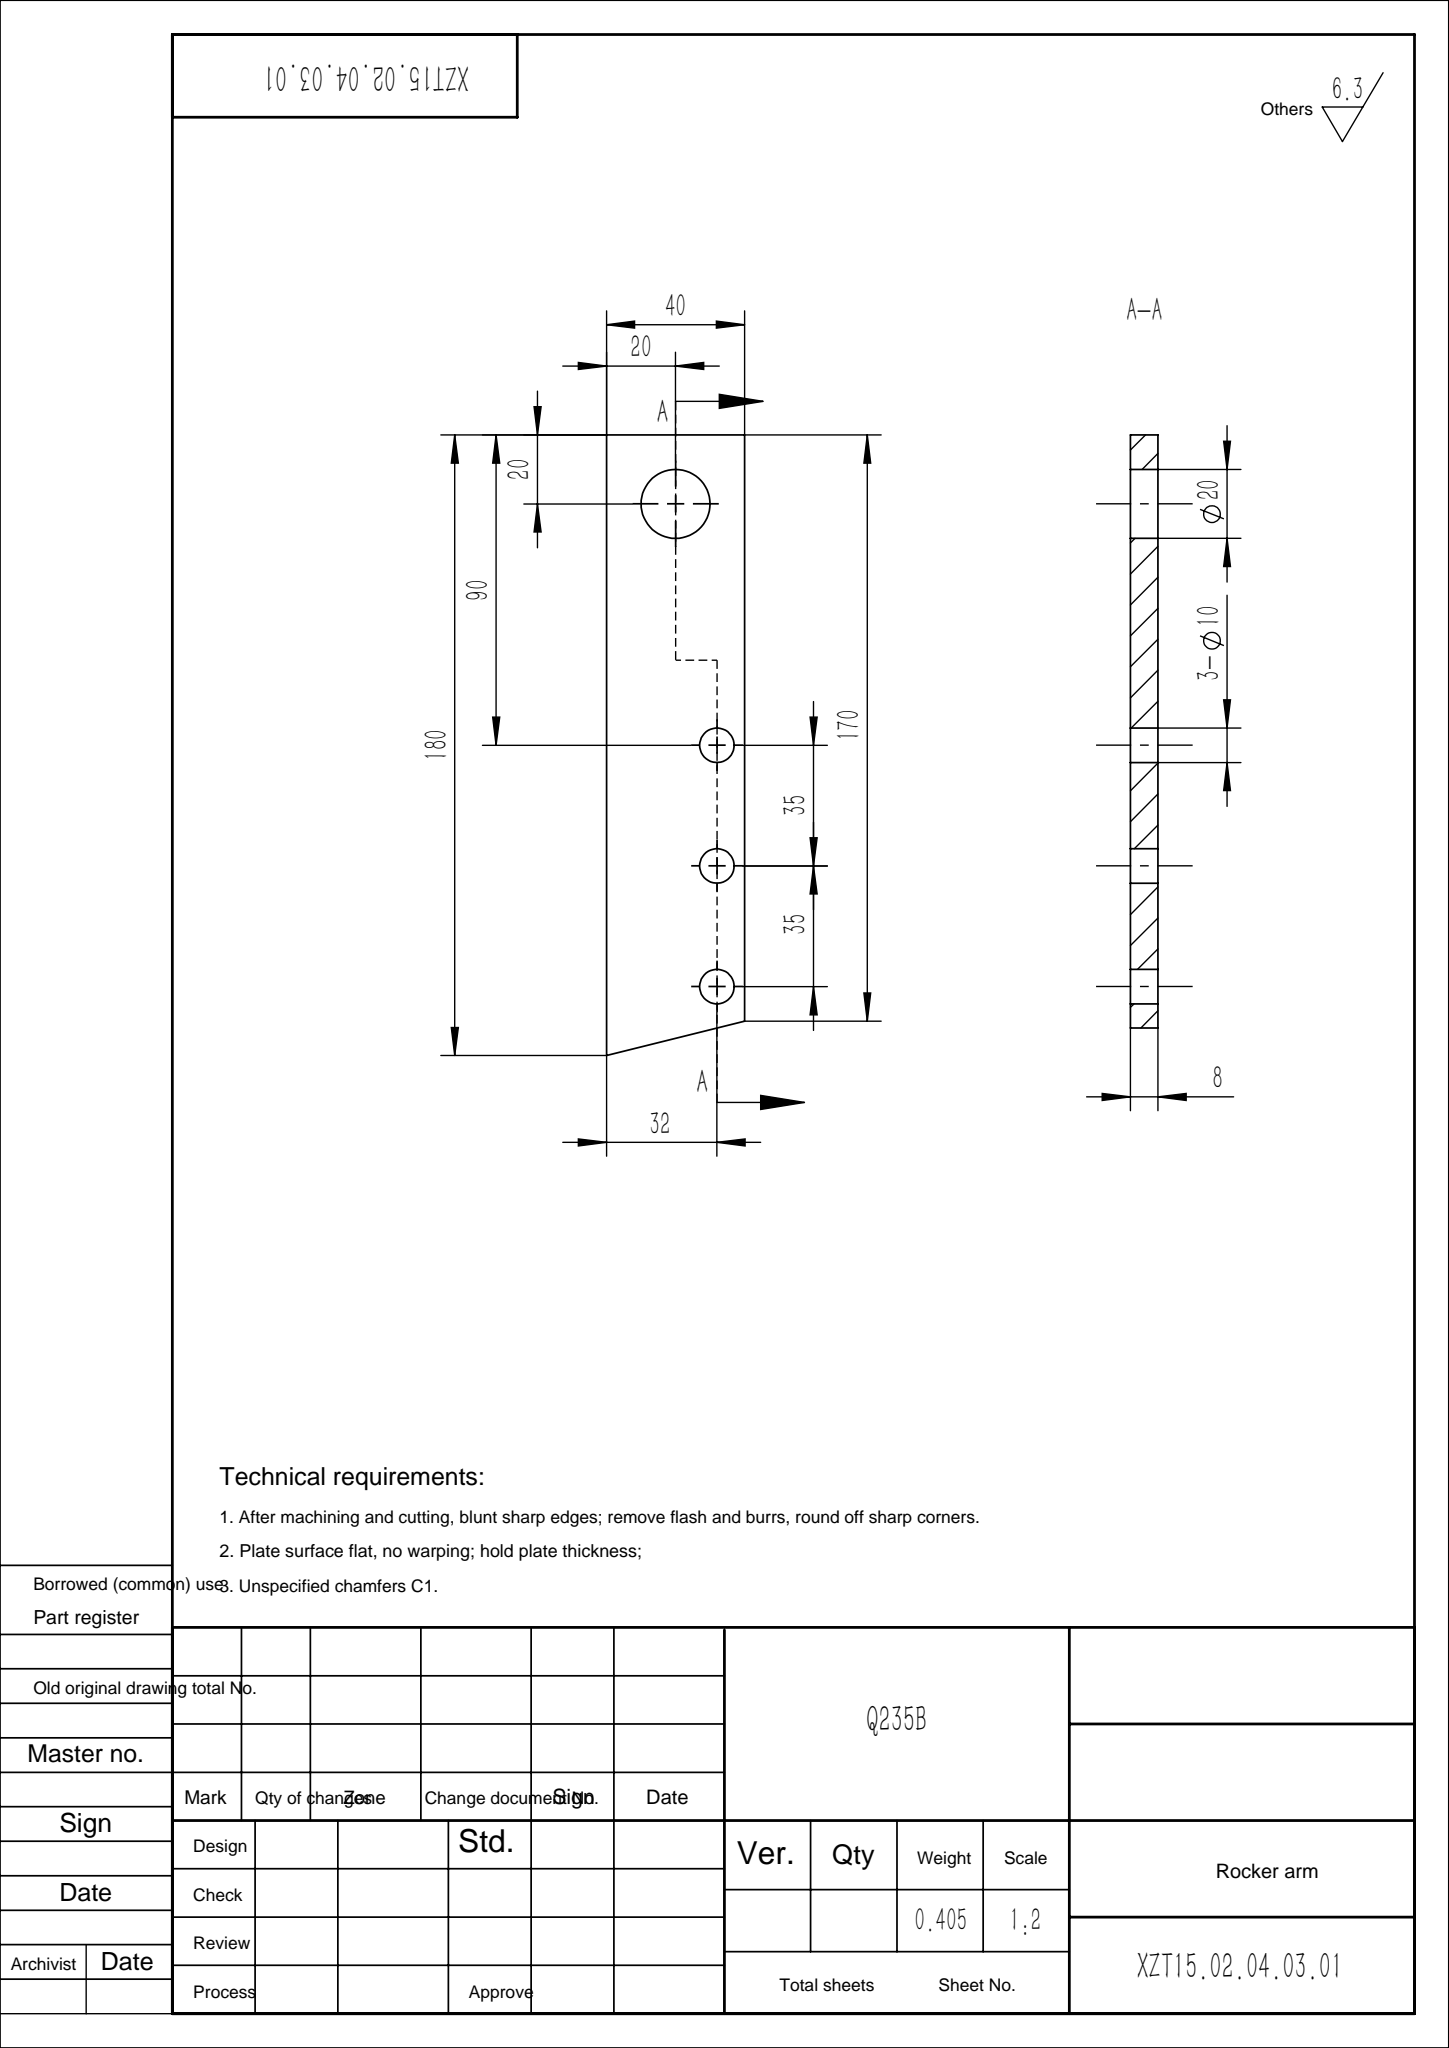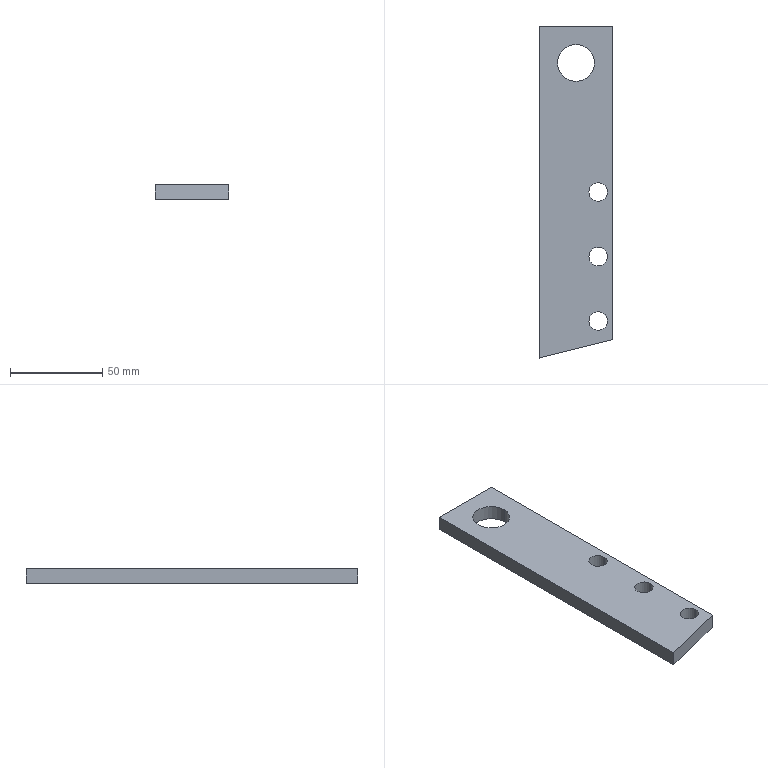Part | SolidWorks | features Extrusion 1 | 1 solid | 14 faces | box 40 x 180 x 8 mm | volume 51602 mm3 | cylinder 8 | plane 6 | commonest cylinder face diameters 10 x6 20 x2
STEP:
#1=CARTESIAN_POINT('',(27.,20.,4.));
#2=VERTEX_POINT('',#1);
#3=CARTESIAN_POINT('',(37.,20.,4.));
#4=VERTEX_POINT('',#3);
#5=CARTESIAN_POINT('',(32.,20.,4.));
#6=DIRECTION('',(0.,0.,1.));
#7=DIRECTION('',(1.,0.,0.));
#8=AXIS2_PLACEMENT_3D('',#5,#6,#7);
#9=CIRCLE('',#8,5.);
#10=EDGE_CURVE('',#2,#4,#9,.T.);
#11=ORIENTED_EDGE('',*,*,#10,.T.);
#12=CARTESIAN_POINT('',(37.,20.,-4.));
#13=VERTEX_POINT('',#12);
#14=CARTESIAN_POINT('',(37.,20.,4.));
#15=DIRECTION('',(0.,0.,-1.));
#16=VECTOR('',#15,1000.);
#17=LINE('',#14,#16);
#18=EDGE_CURVE('',#4,#13,#17,.T.);
#19=ORIENTED_EDGE('',*,*,#18,.T.);
#20=CARTESIAN_POINT('',(27.,20.,-4.));
#21=VERTEX_POINT('',#20);
#22=CARTESIAN_POINT('',(32.,20.,-4.));
#23=DIRECTION('',(0.,0.,1.));
#24=DIRECTION('',(1.,0.,0.));
#25=AXIS2_PLACEMENT_3D('',#22,#23,#24);
#26=CIRCLE('',#25,5.);
#27=EDGE_CURVE('',#21,#13,#26,.T.);
#28=ORIENTED_EDGE('',*,*,#27,.F.);
#29=CARTESIAN_POINT('',(27.,20.,4.));
#30=DIRECTION('',(0.,0.,-1.));
#31=VECTOR('',#30,1000.);
#32=LINE('',#29,#31);
#33=EDGE_CURVE('',#2,#21,#32,.T.);
#34=ORIENTED_EDGE('',*,*,#33,.F.);
#35=EDGE_LOOP('',(#11,#19,#28,#34));
#36=FACE_OUTER_BOUND('',#35,.T.);
#37=CARTESIAN_POINT('',(32.,20.,4.));
#38=DIRECTION('',(0.,0.,-1.));
#39=DIRECTION('',(-1.,0.,0.));
#40=AXIS2_PLACEMENT_3D('',#37,#38,#39);
#41=CYLINDRICAL_SURFACE('',#40,5.);
#42=ADVANCED_FACE('',(#36),#41,.F.);
#43=CARTESIAN_POINT('',(27.,55.,4.));
#44=VERTEX_POINT('',#43);
#45=CARTESIAN_POINT('',(37.,55.,4.));
#46=VERTEX_POINT('',#45);
#47=CARTESIAN_POINT('',(32.,55.,4.));
#48=DIRECTION('',(0.,0.,1.));
#49=DIRECTION('',(1.,0.,0.));
#50=AXIS2_PLACEMENT_3D('',#47,#48,#49);
#51=CIRCLE('',#50,5.);
#52=EDGE_CURVE('',#44,#46,#51,.T.);
#53=ORIENTED_EDGE('',*,*,#52,.T.);
#54=CARTESIAN_POINT('',(37.,55.,-4.));
#55=VERTEX_POINT('',#54);
#56=CARTESIAN_POINT('',(37.,55.,4.));
#57=DIRECTION('',(0.,0.,-1.));
#58=VECTOR('',#57,1000.);
#59=LINE('',#56,#58);
#60=EDGE_CURVE('',#46,#55,#59,.T.);
#61=ORIENTED_EDGE('',*,*,#60,.T.);
#62=CARTESIAN_POINT('',(27.,55.,-4.));
#63=VERTEX_POINT('',#62);
#64=CARTESIAN_POINT('',(32.,55.,-4.));
#65=DIRECTION('',(0.,0.,1.));
#66=DIRECTION('',(1.,0.,0.));
#67=AXIS2_PLACEMENT_3D('',#64,#65,#66);
#68=CIRCLE('',#67,5.);
#69=EDGE_CURVE('',#63,#55,#68,.T.);
#70=ORIENTED_EDGE('',*,*,#69,.F.);
#71=CARTESIAN_POINT('',(27.,55.,4.));
#72=DIRECTION('',(0.,0.,-1.));
#73=VECTOR('',#72,1000.);
#74=LINE('',#71,#73);
#75=EDGE_CURVE('',#44,#63,#74,.T.);
#76=ORIENTED_EDGE('',*,*,#75,.F.);
#77=EDGE_LOOP('',(#53,#61,#70,#76));
#78=FACE_OUTER_BOUND('',#77,.T.);
#79=CARTESIAN_POINT('',(32.,55.,4.));
#80=DIRECTION('',(0.,0.,-1.));
#81=DIRECTION('',(-1.,0.,0.));
#82=AXIS2_PLACEMENT_3D('',#79,#80,#81);
#83=CYLINDRICAL_SURFACE('',#82,5.);
#84=ADVANCED_FACE('',(#78),#83,.F.);
#85=CARTESIAN_POINT('',(27.,90.,4.));
#86=VERTEX_POINT('',#85);
#87=CARTESIAN_POINT('',(37.,90.,4.));
#88=VERTEX_POINT('',#87);
#89=CARTESIAN_POINT('',(32.,90.,4.));
#90=DIRECTION('',(0.,0.,1.));
#91=DIRECTION('',(1.,0.,0.));
#92=AXIS2_PLACEMENT_3D('',#89,#90,#91);
#93=CIRCLE('',#92,5.);
#94=EDGE_CURVE('',#86,#88,#93,.T.);
#95=ORIENTED_EDGE('',*,*,#94,.T.);
#96=CARTESIAN_POINT('',(37.,90.,-4.));
#97=VERTEX_POINT('',#96);
#98=CARTESIAN_POINT('',(37.,90.,4.));
#99=DIRECTION('',(0.,0.,-1.));
#100=VECTOR('',#99,1000.);
#101=LINE('',#98,#100);
#102=EDGE_CURVE('',#88,#97,#101,.T.);
#103=ORIENTED_EDGE('',*,*,#102,.T.);
#104=CARTESIAN_POINT('',(27.,90.,-4.));
#105=VERTEX_POINT('',#104);
#106=CARTESIAN_POINT('',(32.,90.,-4.));
#107=DIRECTION('',(0.,0.,1.));
#108=DIRECTION('',(1.,0.,0.));
#109=AXIS2_PLACEMENT_3D('',#106,#107,#108);
#110=CIRCLE('',#109,5.);
#111=EDGE_CURVE('',#105,#97,#110,.T.);
#112=ORIENTED_EDGE('',*,*,#111,.F.);
#113=CARTESIAN_POINT('',(27.,90.,4.));
#114=DIRECTION('',(0.,0.,-1.));
#115=VECTOR('',#114,1000.);
#116=LINE('',#113,#115);
#117=EDGE_CURVE('',#86,#105,#116,.T.);
#118=ORIENTED_EDGE('',*,*,#117,.F.);
#119=EDGE_LOOP('',(#95,#103,#112,#118));
#120=FACE_OUTER_BOUND('',#119,.T.);
#121=CARTESIAN_POINT('',(32.,90.,4.));
#122=DIRECTION('',(0.,0.,-1.));
#123=DIRECTION('',(-1.,0.,0.));
#124=AXIS2_PLACEMENT_3D('',#121,#122,#123);
#125=CYLINDRICAL_SURFACE('',#124,5.);
#126=ADVANCED_FACE('',(#120),#125,.F.);
#127=CARTESIAN_POINT('',(10.,160.,4.));
#128=VERTEX_POINT('',#127);
#129=CARTESIAN_POINT('',(30.,160.,4.));
#130=VERTEX_POINT('',#129);
#131=CARTESIAN_POINT('',(20.,160.,4.));
#132=DIRECTION('',(0.,0.,1.));
#133=DIRECTION('',(1.,0.,0.));
#134=AXIS2_PLACEMENT_3D('',#131,#132,#133);
#135=CIRCLE('',#134,10.);
#136=EDGE_CURVE('',#128,#130,#135,.T.);
#137=ORIENTED_EDGE('',*,*,#136,.T.);
#138=CARTESIAN_POINT('',(30.,160.,-4.));
#139=VERTEX_POINT('',#138);
#140=CARTESIAN_POINT('',(30.,160.,4.));
#141=DIRECTION('',(0.,0.,-1.));
#142=VECTOR('',#141,1000.);
#143=LINE('',#140,#142);
#144=EDGE_CURVE('',#130,#139,#143,.T.);
#145=ORIENTED_EDGE('',*,*,#144,.T.);
#146=CARTESIAN_POINT('',(10.,160.,-4.));
#147=VERTEX_POINT('',#146);
#148=CARTESIAN_POINT('',(20.,160.,-4.));
#149=DIRECTION('',(0.,0.,1.));
#150=DIRECTION('',(1.,0.,0.));
#151=AXIS2_PLACEMENT_3D('',#148,#149,#150);
#152=CIRCLE('',#151,10.);
#153=EDGE_CURVE('',#147,#139,#152,.T.);
#154=ORIENTED_EDGE('',*,*,#153,.F.);
#155=CARTESIAN_POINT('',(10.,160.,4.));
#156=DIRECTION('',(0.,0.,-1.));
#157=VECTOR('',#156,1000.);
#158=LINE('',#155,#157);
#159=EDGE_CURVE('',#128,#147,#158,.T.);
#160=ORIENTED_EDGE('',*,*,#159,.F.);
#161=EDGE_LOOP('',(#137,#145,#154,#160));
#162=FACE_OUTER_BOUND('',#161,.T.);
#163=CARTESIAN_POINT('',(20.,160.,4.));
#164=DIRECTION('',(0.,0.,-1.));
#165=DIRECTION('',(-1.,0.,0.));
#166=AXIS2_PLACEMENT_3D('',#163,#164,#165);
#167=CYLINDRICAL_SURFACE('',#166,10.);
#168=ADVANCED_FACE('',(#162),#167,.F.);
#169=CARTESIAN_POINT('',(0.,0.,4.));
#170=VERTEX_POINT('',#169);
#171=CARTESIAN_POINT('',(40.,10.,4.));
#172=VERTEX_POINT('',#171);
#173=CARTESIAN_POINT('',(40.,10.,4.));
#174=DIRECTION('',(0.9701,0.2425,0.));
#175=VECTOR('',#174,1000.);
#176=LINE('',#173,#175);
#177=EDGE_CURVE('',#170,#172,#176,.T.);
#178=ORIENTED_EDGE('',*,*,#177,.T.);
#179=CARTESIAN_POINT('',(40.,180.,4.));
#180=VERTEX_POINT('',#179);
#181=CARTESIAN_POINT('',(40.,180.,4.));
#182=DIRECTION('',(0.,1.,0.));
#183=VECTOR('',#182,1000.);
#184=LINE('',#181,#183);
#185=EDGE_CURVE('',#172,#180,#184,.T.);
#186=ORIENTED_EDGE('',*,*,#185,.T.);
#187=CARTESIAN_POINT('',(0.,180.,4.));
#188=VERTEX_POINT('',#187);
#189=CARTESIAN_POINT('',(0.,180.,4.));
#190=DIRECTION('',(-1.,0.,0.));
#191=VECTOR('',#190,1000.);
#192=LINE('',#189,#191);
#193=EDGE_CURVE('',#180,#188,#192,.T.);
#194=ORIENTED_EDGE('',*,*,#193,.T.);
#195=CARTESIAN_POINT('',(0.,0.,4.));
#196=DIRECTION('',(0.,-1.,0.));
#197=VECTOR('',#196,1000.);
#198=LINE('',#195,#197);
#199=EDGE_CURVE('',#188,#170,#198,.T.);
#200=ORIENTED_EDGE('',*,*,#199,.T.);
#201=EDGE_LOOP('',(#178,#186,#194,#200));
#202=FACE_OUTER_BOUND('',#201,.T.);
#203=ORIENTED_EDGE('',*,*,#136,.F.);
#204=CARTESIAN_POINT('',(20.,160.,4.));
#205=DIRECTION('',(0.,0.,1.));
#206=DIRECTION('',(1.,0.,0.));
#207=AXIS2_PLACEMENT_3D('',#204,#205,#206);
#208=CIRCLE('',#207,10.);
#209=EDGE_CURVE('',#130,#128,#208,.T.);
#210=ORIENTED_EDGE('',*,*,#209,.F.);
#211=EDGE_LOOP('',(#203,#210));
#212=FACE_BOUND('',#211,.T.);
#213=ORIENTED_EDGE('',*,*,#94,.F.);
#214=CARTESIAN_POINT('',(32.,90.,4.));
#215=DIRECTION('',(0.,0.,1.));
#216=DIRECTION('',(1.,0.,0.));
#217=AXIS2_PLACEMENT_3D('',#214,#215,#216);
#218=CIRCLE('',#217,5.);
#219=EDGE_CURVE('',#88,#86,#218,.T.);
#220=ORIENTED_EDGE('',*,*,#219,.F.);
#221=EDGE_LOOP('',(#213,#220));
#222=FACE_BOUND('',#221,.T.);
#223=ORIENTED_EDGE('',*,*,#52,.F.);
#224=CARTESIAN_POINT('',(32.,55.,4.));
#225=DIRECTION('',(0.,0.,1.));
#226=DIRECTION('',(1.,0.,0.));
#227=AXIS2_PLACEMENT_3D('',#224,#225,#226);
#228=CIRCLE('',#227,5.);
#229=EDGE_CURVE('',#46,#44,#228,.T.);
#230=ORIENTED_EDGE('',*,*,#229,.F.);
#231=EDGE_LOOP('',(#223,#230));
#232=FACE_BOUND('',#231,.T.);
#233=ORIENTED_EDGE('',*,*,#10,.F.);
#234=CARTESIAN_POINT('',(32.,20.,4.));
#235=DIRECTION('',(0.,0.,1.));
#236=DIRECTION('',(1.,0.,0.));
#237=AXIS2_PLACEMENT_3D('',#234,#235,#236);
#238=CIRCLE('',#237,5.);
#239=EDGE_CURVE('',#4,#2,#238,.T.);
#240=ORIENTED_EDGE('',*,*,#239,.F.);
#241=EDGE_LOOP('',(#233,#240));
#242=FACE_BOUND('',#241,.T.);
#243=CARTESIAN_POINT('',(0.,0.,4.));
#244=DIRECTION('',(0.,0.,-1.));
#245=DIRECTION('',(-1.,0.,0.));
#246=AXIS2_PLACEMENT_3D('',#243,#244,#245);
#247=PLANE('',#246);
#248=ADVANCED_FACE('',(#202,#212,#222,#232,#242),#247,.F.);
#249=ORIENTED_EDGE('',*,*,#69,.T.);
#250=CARTESIAN_POINT('',(32.,55.,-4.));
#251=DIRECTION('',(0.,0.,1.));
#252=DIRECTION('',(1.,0.,0.));
#253=AXIS2_PLACEMENT_3D('',#250,#251,#252);
#254=CIRCLE('',#253,5.);
#255=EDGE_CURVE('',#55,#63,#254,.T.);
#256=ORIENTED_EDGE('',*,*,#255,.T.);
#257=EDGE_LOOP('',(#249,#256));
#258=FACE_BOUND('',#257,.T.);
#259=ORIENTED_EDGE('',*,*,#153,.T.);
#260=CARTESIAN_POINT('',(20.,160.,-4.));
#261=DIRECTION('',(0.,0.,1.));
#262=DIRECTION('',(1.,0.,0.));
#263=AXIS2_PLACEMENT_3D('',#260,#261,#262);
#264=CIRCLE('',#263,10.);
#265=EDGE_CURVE('',#139,#147,#264,.T.);
#266=ORIENTED_EDGE('',*,*,#265,.T.);
#267=EDGE_LOOP('',(#259,#266));
#268=FACE_BOUND('',#267,.T.);
#269=CARTESIAN_POINT('',(0.,0.,-4.));
#270=VERTEX_POINT('',#269);
#271=CARTESIAN_POINT('',(40.,10.,-4.));
#272=VERTEX_POINT('',#271);
#273=CARTESIAN_POINT('',(40.,10.,-4.));
#274=DIRECTION('',(0.9701,0.2425,0.));
#275=VECTOR('',#274,1000.);
#276=LINE('',#273,#275);
#277=EDGE_CURVE('',#270,#272,#276,.T.);
#278=ORIENTED_EDGE('',*,*,#277,.F.);
#279=CARTESIAN_POINT('',(0.,180.,-4.));
#280=VERTEX_POINT('',#279);
#281=CARTESIAN_POINT('',(0.,0.,-4.));
#282=DIRECTION('',(0.,-1.,0.));
#283=VECTOR('',#282,1000.);
#284=LINE('',#281,#283);
#285=EDGE_CURVE('',#280,#270,#284,.T.);
#286=ORIENTED_EDGE('',*,*,#285,.F.);
#287=CARTESIAN_POINT('',(40.,180.,-4.));
#288=VERTEX_POINT('',#287);
#289=CARTESIAN_POINT('',(0.,180.,-4.));
#290=DIRECTION('',(-1.,0.,0.));
#291=VECTOR('',#290,1000.);
#292=LINE('',#289,#291);
#293=EDGE_CURVE('',#288,#280,#292,.T.);
#294=ORIENTED_EDGE('',*,*,#293,.F.);
#295=CARTESIAN_POINT('',(40.,180.,-4.));
#296=DIRECTION('',(0.,1.,0.));
#297=VECTOR('',#296,1000.);
#298=LINE('',#295,#297);
#299=EDGE_CURVE('',#272,#288,#298,.T.);
#300=ORIENTED_EDGE('',*,*,#299,.F.);
#301=EDGE_LOOP('',(#278,#286,#294,#300));
#302=FACE_OUTER_BOUND('',#301,.T.);
#303=ORIENTED_EDGE('',*,*,#111,.T.);
#304=CARTESIAN_POINT('',(32.,90.,-4.));
#305=DIRECTION('',(0.,0.,1.));
#306=DIRECTION('',(1.,0.,0.));
#307=AXIS2_PLACEMENT_3D('',#304,#305,#306);
#308=CIRCLE('',#307,5.);
#309=EDGE_CURVE('',#97,#105,#308,.T.);
#310=ORIENTED_EDGE('',*,*,#309,.T.);
#311=EDGE_LOOP('',(#303,#310));
#312=FACE_BOUND('',#311,.T.);
#313=ORIENTED_EDGE('',*,*,#27,.T.);
#314=CARTESIAN_POINT('',(32.,20.,-4.));
#315=DIRECTION('',(0.,0.,1.));
#316=DIRECTION('',(1.,0.,0.));
#317=AXIS2_PLACEMENT_3D('',#314,#315,#316);
#318=CIRCLE('',#317,5.);
#319=EDGE_CURVE('',#13,#21,#318,.T.);
#320=ORIENTED_EDGE('',*,*,#319,.T.);
#321=EDGE_LOOP('',(#313,#320));
#322=FACE_BOUND('',#321,.T.);
#323=CARTESIAN_POINT('',(0.,0.,-4.));
#324=DIRECTION('',(0.,0.,-1.));
#325=DIRECTION('',(-1.,0.,0.));
#326=AXIS2_PLACEMENT_3D('',#323,#324,#325);
#327=PLANE('',#326);
#328=ADVANCED_FACE('',(#258,#268,#302,#312,#322),#327,.T.);
#329=ORIENTED_EDGE('',*,*,#277,.T.);
#330=CARTESIAN_POINT('',(40.,10.,4.));
#331=DIRECTION('',(0.,0.,-1.));
#332=VECTOR('',#331,1000.);
#333=LINE('',#330,#332);
#334=EDGE_CURVE('',#172,#272,#333,.T.);
#335=ORIENTED_EDGE('',*,*,#334,.F.);
#336=ORIENTED_EDGE('',*,*,#177,.F.);
#337=CARTESIAN_POINT('',(0.,0.,4.));
#338=DIRECTION('',(0.,0.,-1.));
#339=VECTOR('',#338,1000.);
#340=LINE('',#337,#339);
#341=EDGE_CURVE('',#170,#270,#340,.T.);
#342=ORIENTED_EDGE('',*,*,#341,.T.);
#343=EDGE_LOOP('',(#329,#335,#336,#342));
#344=FACE_OUTER_BOUND('',#343,.T.);
#345=CARTESIAN_POINT('',(40.,10.,4.));
#346=DIRECTION('',(-0.2425,0.9701,0.));
#347=DIRECTION('',(-0.9701,-0.2425,0.));
#348=AXIS2_PLACEMENT_3D('',#345,#346,#347);
#349=PLANE('',#348);
#350=ADVANCED_FACE('',(#344),#349,.F.);
#351=ORIENTED_EDGE('',*,*,#299,.T.);
#352=CARTESIAN_POINT('',(40.,180.,4.));
#353=DIRECTION('',(0.,0.,-1.));
#354=VECTOR('',#353,1000.);
#355=LINE('',#352,#354);
#356=EDGE_CURVE('',#180,#288,#355,.T.);
#357=ORIENTED_EDGE('',*,*,#356,.F.);
#358=ORIENTED_EDGE('',*,*,#185,.F.);
#359=ORIENTED_EDGE('',*,*,#334,.T.);
#360=EDGE_LOOP('',(#351,#357,#358,#359));
#361=FACE_OUTER_BOUND('',#360,.T.);
#362=CARTESIAN_POINT('',(40.,180.,4.));
#363=DIRECTION('',(-1.,0.,0.));
#364=DIRECTION('',(0.,-1.,0.));
#365=AXIS2_PLACEMENT_3D('',#362,#363,#364);
#366=PLANE('',#365);
#367=ADVANCED_FACE('',(#361),#366,.F.);
#368=ORIENTED_EDGE('',*,*,#293,.T.);
#369=CARTESIAN_POINT('',(0.,180.,4.));
#370=DIRECTION('',(0.,0.,-1.));
#371=VECTOR('',#370,1000.);
#372=LINE('',#369,#371);
#373=EDGE_CURVE('',#188,#280,#372,.T.);
#374=ORIENTED_EDGE('',*,*,#373,.F.);
#375=ORIENTED_EDGE('',*,*,#193,.F.);
#376=ORIENTED_EDGE('',*,*,#356,.T.);
#377=EDGE_LOOP('',(#368,#374,#375,#376));
#378=FACE_OUTER_BOUND('',#377,.T.);
#379=CARTESIAN_POINT('',(0.,180.,4.));
#380=DIRECTION('',(0.,-1.,0.));
#381=DIRECTION('',(0.,0.,-1.));
#382=AXIS2_PLACEMENT_3D('',#379,#380,#381);
#383=PLANE('',#382);
#384=ADVANCED_FACE('',(#378),#383,.F.);
#385=ORIENTED_EDGE('',*,*,#285,.T.);
#386=ORIENTED_EDGE('',*,*,#341,.F.);
#387=ORIENTED_EDGE('',*,*,#199,.F.);
#388=ORIENTED_EDGE('',*,*,#373,.T.);
#389=EDGE_LOOP('',(#385,#386,#387,#388));
#390=FACE_OUTER_BOUND('',#389,.T.);
#391=CARTESIAN_POINT('',(0.,0.,4.));
#392=DIRECTION('',(1.,0.,0.));
#393=DIRECTION('',(0.,0.,-1.));
#394=AXIS2_PLACEMENT_3D('',#391,#392,#393);
#395=PLANE('',#394);
#396=ADVANCED_FACE('',(#390),#395,.F.);
#397=ORIENTED_EDGE('',*,*,#144,.F.);
#398=ORIENTED_EDGE('',*,*,#209,.T.);
#399=ORIENTED_EDGE('',*,*,#159,.T.);
#400=ORIENTED_EDGE('',*,*,#265,.F.);
#401=EDGE_LOOP('',(#397,#398,#399,#400));
#402=FACE_OUTER_BOUND('',#401,.T.);
#403=CARTESIAN_POINT('',(20.,160.,4.));
#404=DIRECTION('',(0.,0.,-1.));
#405=DIRECTION('',(-1.,0.,0.));
#406=AXIS2_PLACEMENT_3D('',#403,#404,#405);
#407=CYLINDRICAL_SURFACE('',#406,10.);
#408=ADVANCED_FACE('',(#402),#407,.F.);
#409=ORIENTED_EDGE('',*,*,#102,.F.);
#410=ORIENTED_EDGE('',*,*,#219,.T.);
#411=ORIENTED_EDGE('',*,*,#117,.T.);
#412=ORIENTED_EDGE('',*,*,#309,.F.);
#413=EDGE_LOOP('',(#409,#410,#411,#412));
#414=FACE_OUTER_BOUND('',#413,.T.);
#415=CARTESIAN_POINT('',(32.,90.,4.));
#416=DIRECTION('',(0.,0.,-1.));
#417=DIRECTION('',(-1.,0.,0.));
#418=AXIS2_PLACEMENT_3D('',#415,#416,#417);
#419=CYLINDRICAL_SURFACE('',#418,5.);
#420=ADVANCED_FACE('',(#414),#419,.F.);
#421=ORIENTED_EDGE('',*,*,#60,.F.);
#422=ORIENTED_EDGE('',*,*,#229,.T.);
#423=ORIENTED_EDGE('',*,*,#75,.T.);
#424=ORIENTED_EDGE('',*,*,#255,.F.);
#425=EDGE_LOOP('',(#421,#422,#423,#424));
#426=FACE_OUTER_BOUND('',#425,.T.);
#427=CARTESIAN_POINT('',(32.,55.,4.));
#428=DIRECTION('',(0.,0.,-1.));
#429=DIRECTION('',(-1.,0.,0.));
#430=AXIS2_PLACEMENT_3D('',#427,#428,#429);
#431=CYLINDRICAL_SURFACE('',#430,5.);
#432=ADVANCED_FACE('',(#426),#431,.F.);
#433=ORIENTED_EDGE('',*,*,#18,.F.);
#434=ORIENTED_EDGE('',*,*,#239,.T.);
#435=ORIENTED_EDGE('',*,*,#33,.T.);
#436=ORIENTED_EDGE('',*,*,#319,.F.);
#437=EDGE_LOOP('',(#433,#434,#435,#436));
#438=FACE_OUTER_BOUND('',#437,.T.);
#439=CARTESIAN_POINT('',(32.,20.,4.));
#440=DIRECTION('',(0.,0.,-1.));
#441=DIRECTION('',(-1.,0.,0.));
#442=AXIS2_PLACEMENT_3D('',#439,#440,#441);
#443=CYLINDRICAL_SURFACE('',#442,5.);
#444=ADVANCED_FACE('',(#438),#443,.F.);
#445=CLOSED_SHELL('',(#42,#84,#126,#168,#248,#328,#350,#367,#384,#396,#408,#420,#432,#444));
#446=MANIFOLD_SOLID_BREP('',#445);
#447=CARTESIAN_POINT('',(0.,0.,0.));
#448=DIRECTION('',(0.,0.,1.));
#449=DIRECTION('',(1.,0.,0.));
#450=AXIS2_PLACEMENT_3D('',#447,#448,#449);
#451=(LENGTH_UNIT()NAMED_UNIT(*)SI_UNIT(.MILLI.,.METRE.));
#452=UNCERTAINTY_MEASURE_WITH_UNIT(LENGTH_MEASURE(0.00001),#451,'','');
#453=(NAMED_UNIT(*)PLANE_ANGLE_UNIT()SI_UNIT($,.RADIAN.));
#454=(NAMED_UNIT(*)SI_UNIT($,.STERADIAN.)SOLID_ANGLE_UNIT());
#455=(GEOMETRIC_REPRESENTATION_CONTEXT(3)GLOBAL_UNCERTAINTY_ASSIGNED_CONTEXT((#452))GLOBAL_UNIT_ASSIGNED_CONTEXT((#451,#453,#454))REPRESENTATION_CONTEXT('',''));
#456=ADVANCED_BREP_SHAPE_REPRESENTATION('',(#446,#450),#455);